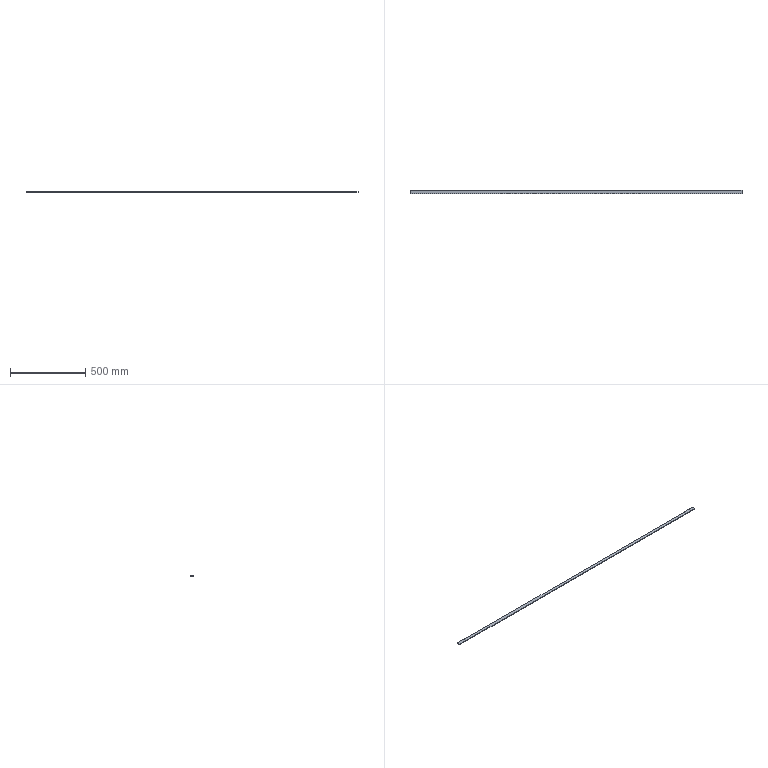Part | SolidWorks | features Chamfer 1, Extrusion 1, Fillet 1, ICE 1 | 1 solid | 12 faces | box 2200 x 24 x 4 mm | volume 178062 mm3 | plane 8 | cylinder 4 | commonest cylinder face diameters 4 x4
STEP:
#1=CARTESIAN_POINT('',(1030.,24.,0.));
#2=VERTEX_POINT('',#1);
#3=CARTESIAN_POINT('',(1100.,24.,0.));
#4=VERTEX_POINT('',#3);
#5=CARTESIAN_POINT('',(1100.,24.,0.));
#6=DIRECTION('',(1.,0.,0.));
#7=VECTOR('',#6,1000.);
#8=LINE('',#5,#7);
#9=EDGE_CURVE('',#2,#4,#8,.T.);
#10=ORIENTED_EDGE('',*,*,#9,.F.);
#11=CARTESIAN_POINT('',(1028.,22.,2.));
#12=VERTEX_POINT('',#11);
#13=CARTESIAN_POINT('',(1030.,24.,0.));
#14=CARTESIAN_POINT('',(1030.,24.,1.172));
#15=CARTESIAN_POINT('',(1029.172,23.172,2.));
#16=CARTESIAN_POINT('',(1028.,22.,2.));
#17=(BOUNDED_CURVE()B_SPLINE_CURVE(3,(#13,#14,#15,#16),.UNSPECIFIED.,.F.,.F.)B_SPLINE_CURVE_WITH_KNOTS((4,4),(3.142,4.712),.UNSPECIFIED.)CURVE()GEOMETRIC_REPRESENTATION_ITEM()RATIONAL_B_SPLINE_CURVE((1.,0.8047,0.8047,1.))REPRESENTATION_ITEM(''));
#18=EDGE_CURVE('',#2,#12,#17,.T.);
#19=ORIENTED_EDGE('',*,*,#18,.T.);
#20=CARTESIAN_POINT('',(1100.,22.,2.));
#21=VERTEX_POINT('',#20);
#22=CARTESIAN_POINT('',(-1100.,22.,2.));
#23=DIRECTION('',(-1.,0.,0.));
#24=VECTOR('',#23,1000.);
#25=LINE('',#22,#24);
#26=EDGE_CURVE('',#21,#12,#25,.T.);
#27=ORIENTED_EDGE('',*,*,#26,.F.);
#28=CARTESIAN_POINT('',(1100.,22.,0.));
#29=DIRECTION('',(1.,0.,0.));
#30=DIRECTION('',(0.,0.,1.));
#31=AXIS2_PLACEMENT_3D('',#28,#29,#30);
#32=CIRCLE('',#31,2.);
#33=EDGE_CURVE('',#4,#21,#32,.T.);
#34=ORIENTED_EDGE('',*,*,#33,.F.);
#35=EDGE_LOOP('',(#10,#19,#27,#34));
#36=FACE_OUTER_BOUND('',#35,.T.);
#37=CARTESIAN_POINT('',(0.,22.,0.));
#38=DIRECTION('',(-1.,0.,0.));
#39=DIRECTION('',(0.,0.,1.));
#40=AXIS2_PLACEMENT_3D('',#37,#38,#39);
#41=CYLINDRICAL_SURFACE('',#40,2.);
#42=ADVANCED_FACE('',(#36),#41,.T.);
#43=CARTESIAN_POINT('',(1028.,22.,-2.));
#44=VERTEX_POINT('',#43);
#45=CARTESIAN_POINT('',(1100.,22.,-2.));
#46=VERTEX_POINT('',#45);
#47=CARTESIAN_POINT('',(1100.,22.,-2.));
#48=DIRECTION('',(1.,0.,0.));
#49=VECTOR('',#48,1000.);
#50=LINE('',#47,#49);
#51=EDGE_CURVE('',#44,#46,#50,.T.);
#52=ORIENTED_EDGE('',*,*,#51,.F.);
#53=CARTESIAN_POINT('',(1028.,22.,-2.));
#54=CARTESIAN_POINT('',(1029.172,23.172,-2.));
#55=CARTESIAN_POINT('',(1030.,24.,-1.172));
#56=CARTESIAN_POINT('',(1030.,24.,0.));
#57=(BOUNDED_CURVE()B_SPLINE_CURVE(3,(#53,#54,#55,#56),.UNSPECIFIED.,.F.,.T.)B_SPLINE_CURVE_WITH_KNOTS((4,4),(4.712,6.283),.UNSPECIFIED.)CURVE()GEOMETRIC_REPRESENTATION_ITEM()RATIONAL_B_SPLINE_CURVE((1.,0.8047,0.8047,1.))REPRESENTATION_ITEM(''));
#58=EDGE_CURVE('',#44,#2,#57,.T.);
#59=ORIENTED_EDGE('',*,*,#58,.T.);
#60=ORIENTED_EDGE('',*,*,#9,.T.);
#61=CARTESIAN_POINT('',(1100.,22.,0.));
#62=DIRECTION('',(1.,0.,0.));
#63=DIRECTION('',(0.,0.,1.));
#64=AXIS2_PLACEMENT_3D('',#61,#62,#63);
#65=CIRCLE('',#64,2.);
#66=EDGE_CURVE('',#46,#4,#65,.T.);
#67=ORIENTED_EDGE('',*,*,#66,.F.);
#68=EDGE_LOOP('',(#52,#59,#60,#67));
#69=FACE_OUTER_BOUND('',#68,.T.);
#70=CARTESIAN_POINT('',(0.,22.,0.));
#71=DIRECTION('',(1.,0.,0.));
#72=DIRECTION('',(0.,0.,-1.));
#73=AXIS2_PLACEMENT_3D('',#70,#71,#72);
#74=CYLINDRICAL_SURFACE('',#73,2.);
#75=ADVANCED_FACE('',(#69),#74,.T.);
#76=CARTESIAN_POINT('',(-1100.,22.,2.));
#77=VERTEX_POINT('',#76);
#78=CARTESIAN_POINT('',(-1100.,24.,0.));
#79=VERTEX_POINT('',#78);
#80=CARTESIAN_POINT('',(-1100.,22.,0.));
#81=DIRECTION('',(-1.,0.,0.));
#82=DIRECTION('',(0.,0.,-1.));
#83=AXIS2_PLACEMENT_3D('',#80,#81,#82);
#84=CIRCLE('',#83,2.);
#85=EDGE_CURVE('',#77,#79,#84,.T.);
#86=ORIENTED_EDGE('',*,*,#85,.T.);
#87=CARTESIAN_POINT('',(-1100.,22.,-2.));
#88=VERTEX_POINT('',#87);
#89=CARTESIAN_POINT('',(-1100.,22.,0.));
#90=DIRECTION('',(-1.,0.,0.));
#91=DIRECTION('',(0.,0.,-1.));
#92=AXIS2_PLACEMENT_3D('',#89,#90,#91);
#93=CIRCLE('',#92,2.);
#94=EDGE_CURVE('',#79,#88,#93,.T.);
#95=ORIENTED_EDGE('',*,*,#94,.T.);
#96=CARTESIAN_POINT('',(-1100.,0.,-2.));
#97=VERTEX_POINT('',#96);
#98=CARTESIAN_POINT('',(-1100.,24.,-2.));
#99=DIRECTION('',(0.,-1.,0.));
#100=VECTOR('',#99,1000.);
#101=LINE('',#98,#100);
#102=EDGE_CURVE('',#88,#97,#101,.T.);
#103=ORIENTED_EDGE('',*,*,#102,.T.);
#104=CARTESIAN_POINT('',(-1100.,0.,2.));
#105=VERTEX_POINT('',#104);
#106=CARTESIAN_POINT('',(-1100.,0.,2.));
#107=DIRECTION('',(0.,0.,1.));
#108=VECTOR('',#107,1000.);
#109=LINE('',#106,#108);
#110=EDGE_CURVE('',#97,#105,#109,.T.);
#111=ORIENTED_EDGE('',*,*,#110,.T.);
#112=CARTESIAN_POINT('',(-1100.,24.,2.));
#113=DIRECTION('',(0.,-1.,0.));
#114=VECTOR('',#113,1000.);
#115=LINE('',#112,#114);
#116=EDGE_CURVE('',#77,#105,#115,.T.);
#117=ORIENTED_EDGE('',*,*,#116,.F.);
#118=EDGE_LOOP('',(#86,#95,#103,#111,#117));
#119=FACE_OUTER_BOUND('',#118,.T.);
#120=CARTESIAN_POINT('',(-1100.,24.,2.));
#121=DIRECTION('',(1.,0.,0.));
#122=DIRECTION('',(0.,0.,-1.));
#123=AXIS2_PLACEMENT_3D('',#120,#121,#122);
#124=PLANE('',#123);
#125=ADVANCED_FACE('',(#119),#124,.F.);
#126=ORIENTED_EDGE('',*,*,#26,.T.);
#127=CARTESIAN_POINT('',(1026.,20.,2.));
#128=VERTEX_POINT('',#127);
#129=CARTESIAN_POINT('',(1065.,59.,2.));
#130=DIRECTION('',(-0.7071,-0.7071,0.));
#131=VECTOR('',#130,1000.);
#132=LINE('',#129,#131);
#133=EDGE_CURVE('',#12,#128,#132,.T.);
#134=ORIENTED_EDGE('',*,*,#133,.T.);
#135=CARTESIAN_POINT('',(-1026.,20.,2.));
#136=VERTEX_POINT('',#135);
#137=CARTESIAN_POINT('',(-1030.,20.,2.));
#138=DIRECTION('',(1.,0.,0.));
#139=VECTOR('',#138,1000.);
#140=LINE('',#137,#139);
#141=EDGE_CURVE('',#136,#128,#140,.T.);
#142=ORIENTED_EDGE('',*,*,#141,.F.);
#143=CARTESIAN_POINT('',(-1028.,22.,2.));
#144=VERTEX_POINT('',#143);
#145=CARTESIAN_POINT('',(35.,-1041.,2.));
#146=DIRECTION('',(-0.7071,0.7071,0.));
#147=VECTOR('',#146,1000.);
#148=LINE('',#145,#147);
#149=EDGE_CURVE('',#136,#144,#148,.T.);
#150=ORIENTED_EDGE('',*,*,#149,.T.);
#151=CARTESIAN_POINT('',(-1100.,22.,2.));
#152=DIRECTION('',(-1.,0.,0.));
#153=VECTOR('',#152,1000.);
#154=LINE('',#151,#153);
#155=EDGE_CURVE('',#144,#77,#154,.T.);
#156=ORIENTED_EDGE('',*,*,#155,.T.);
#157=ORIENTED_EDGE('',*,*,#116,.T.);
#158=CARTESIAN_POINT('',(1100.,0.,2.));
#159=VERTEX_POINT('',#158);
#160=CARTESIAN_POINT('',(1100.,0.,2.));
#161=DIRECTION('',(1.,0.,0.));
#162=VECTOR('',#161,1000.);
#163=LINE('',#160,#162);
#164=EDGE_CURVE('',#105,#159,#163,.T.);
#165=ORIENTED_EDGE('',*,*,#164,.T.);
#166=CARTESIAN_POINT('',(1100.,24.,2.));
#167=DIRECTION('',(0.,-1.,0.));
#168=VECTOR('',#167,1000.);
#169=LINE('',#166,#168);
#170=EDGE_CURVE('',#21,#159,#169,.T.);
#171=ORIENTED_EDGE('',*,*,#170,.F.);
#172=EDGE_LOOP('',(#126,#134,#142,#150,#156,#157,#165,#171));
#173=FACE_OUTER_BOUND('',#172,.T.);
#174=CARTESIAN_POINT('',(1100.,24.,2.));
#175=DIRECTION('',(0.,0.,-1.));
#176=DIRECTION('',(-1.,0.,0.));
#177=AXIS2_PLACEMENT_3D('',#174,#175,#176);
#178=PLANE('',#177);
#179=ADVANCED_FACE('',(#173),#178,.F.);
#180=CARTESIAN_POINT('',(1100.,0.,-2.));
#181=VERTEX_POINT('',#180);
#182=CARTESIAN_POINT('',(1100.,24.,-2.));
#183=DIRECTION('',(0.,-1.,0.));
#184=VECTOR('',#183,1000.);
#185=LINE('',#182,#184);
#186=EDGE_CURVE('',#46,#181,#185,.T.);
#187=ORIENTED_EDGE('',*,*,#186,.F.);
#188=ORIENTED_EDGE('',*,*,#66,.T.);
#189=ORIENTED_EDGE('',*,*,#33,.T.);
#190=ORIENTED_EDGE('',*,*,#170,.T.);
#191=CARTESIAN_POINT('',(1100.,0.,2.));
#192=DIRECTION('',(0.,0.,-1.));
#193=VECTOR('',#192,1000.);
#194=LINE('',#191,#193);
#195=EDGE_CURVE('',#159,#181,#194,.T.);
#196=ORIENTED_EDGE('',*,*,#195,.T.);
#197=EDGE_LOOP('',(#187,#188,#189,#190,#196));
#198=FACE_OUTER_BOUND('',#197,.T.);
#199=CARTESIAN_POINT('',(1100.,24.,2.));
#200=DIRECTION('',(-1.,0.,0.));
#201=DIRECTION('',(0.,0.,1.));
#202=AXIS2_PLACEMENT_3D('',#199,#200,#201);
#203=PLANE('',#202);
#204=ADVANCED_FACE('',(#198),#203,.F.);
#205=CARTESIAN_POINT('',(-1028.,22.,-2.));
#206=VERTEX_POINT('',#205);
#207=CARTESIAN_POINT('',(1100.,22.,-2.));
#208=DIRECTION('',(1.,0.,0.));
#209=VECTOR('',#208,1000.);
#210=LINE('',#207,#209);
#211=EDGE_CURVE('',#88,#206,#210,.T.);
#212=ORIENTED_EDGE('',*,*,#211,.T.);
#213=CARTESIAN_POINT('',(-1026.,20.,-2.));
#214=VERTEX_POINT('',#213);
#215=CARTESIAN_POINT('',(35.,-1041.,-2.));
#216=DIRECTION('',(0.7071,-0.7071,0.));
#217=VECTOR('',#216,1000.);
#218=LINE('',#215,#217);
#219=EDGE_CURVE('',#206,#214,#218,.T.);
#220=ORIENTED_EDGE('',*,*,#219,.T.);
#221=CARTESIAN_POINT('',(1026.,20.,-2.));
#222=VERTEX_POINT('',#221);
#223=CARTESIAN_POINT('',(-1030.,20.,-2.));
#224=DIRECTION('',(1.,0.,0.));
#225=VECTOR('',#224,1000.);
#226=LINE('',#223,#225);
#227=EDGE_CURVE('',#214,#222,#226,.T.);
#228=ORIENTED_EDGE('',*,*,#227,.T.);
#229=CARTESIAN_POINT('',(1065.,59.,-2.));
#230=DIRECTION('',(0.7071,0.7071,0.));
#231=VECTOR('',#230,1000.);
#232=LINE('',#229,#231);
#233=EDGE_CURVE('',#222,#44,#232,.T.);
#234=ORIENTED_EDGE('',*,*,#233,.T.);
#235=ORIENTED_EDGE('',*,*,#51,.T.);
#236=ORIENTED_EDGE('',*,*,#186,.T.);
#237=CARTESIAN_POINT('',(1100.,0.,-2.));
#238=DIRECTION('',(-1.,0.,0.));
#239=VECTOR('',#238,1000.);
#240=LINE('',#237,#239);
#241=EDGE_CURVE('',#181,#97,#240,.T.);
#242=ORIENTED_EDGE('',*,*,#241,.T.);
#243=ORIENTED_EDGE('',*,*,#102,.F.);
#244=EDGE_LOOP('',(#212,#220,#228,#234,#235,#236,#242,#243));
#245=FACE_OUTER_BOUND('',#244,.T.);
#246=CARTESIAN_POINT('',(1100.,24.,-2.));
#247=DIRECTION('',(0.,0.,1.));
#248=DIRECTION('',(1.,0.,0.));
#249=AXIS2_PLACEMENT_3D('',#246,#247,#248);
#250=PLANE('',#249);
#251=ADVANCED_FACE('',(#245),#250,.F.);
#252=ORIENTED_EDGE('',*,*,#110,.F.);
#253=ORIENTED_EDGE('',*,*,#241,.F.);
#254=ORIENTED_EDGE('',*,*,#195,.F.);
#255=ORIENTED_EDGE('',*,*,#164,.F.);
#256=EDGE_LOOP('',(#252,#253,#254,#255));
#257=FACE_OUTER_BOUND('',#256,.T.);
#258=CARTESIAN_POINT('',(0.,0.,0.));
#259=DIRECTION('',(0.,1.,0.));
#260=DIRECTION('',(0.,0.,1.));
#261=AXIS2_PLACEMENT_3D('',#258,#259,#260);
#262=PLANE('',#261);
#263=ADVANCED_FACE('',(#257),#262,.F.);
#264=ORIENTED_EDGE('',*,*,#155,.F.);
#265=CARTESIAN_POINT('',(-1030.,24.,0.));
#266=VERTEX_POINT('',#265);
#267=CARTESIAN_POINT('',(-1028.,22.,2.));
#268=CARTESIAN_POINT('',(-1029.172,23.172,2.));
#269=CARTESIAN_POINT('',(-1030.,24.,1.172));
#270=CARTESIAN_POINT('',(-1030.,24.,0.));
#271=(BOUNDED_CURVE()B_SPLINE_CURVE(3,(#267,#268,#269,#270),.UNSPECIFIED.,.F.,.F.)B_SPLINE_CURVE_WITH_KNOTS((4,4),(4.712,6.283),.UNSPECIFIED.)CURVE()GEOMETRIC_REPRESENTATION_ITEM()RATIONAL_B_SPLINE_CURVE((1.,0.8047,0.8047,1.))REPRESENTATION_ITEM(''));
#272=EDGE_CURVE('',#144,#266,#271,.T.);
#273=ORIENTED_EDGE('',*,*,#272,.T.);
#274=CARTESIAN_POINT('',(1100.,24.,0.));
#275=DIRECTION('',(1.,0.,0.));
#276=VECTOR('',#275,1000.);
#277=LINE('',#274,#276);
#278=EDGE_CURVE('',#79,#266,#277,.T.);
#279=ORIENTED_EDGE('',*,*,#278,.F.);
#280=ORIENTED_EDGE('',*,*,#85,.F.);
#281=EDGE_LOOP('',(#264,#273,#279,#280));
#282=FACE_OUTER_BOUND('',#281,.T.);
#283=CARTESIAN_POINT('',(0.,22.,0.));
#284=DIRECTION('',(-1.,0.,0.));
#285=DIRECTION('',(0.,0.,1.));
#286=AXIS2_PLACEMENT_3D('',#283,#284,#285);
#287=CYLINDRICAL_SURFACE('',#286,2.);
#288=ADVANCED_FACE('',(#282),#287,.T.);
#289=ORIENTED_EDGE('',*,*,#278,.T.);
#290=CARTESIAN_POINT('',(-1030.,24.,0.));
#291=CARTESIAN_POINT('',(-1030.,24.,-1.172));
#292=CARTESIAN_POINT('',(-1029.172,23.172,-2.));
#293=CARTESIAN_POINT('',(-1028.,22.,-2.));
#294=(BOUNDED_CURVE()B_SPLINE_CURVE(3,(#290,#291,#292,#293),.UNSPECIFIED.,.F.,.F.)B_SPLINE_CURVE_WITH_KNOTS((4,4),(3.142,4.712),.UNSPECIFIED.)CURVE()GEOMETRIC_REPRESENTATION_ITEM()RATIONAL_B_SPLINE_CURVE((1.,0.8047,0.8047,1.))REPRESENTATION_ITEM(''));
#295=EDGE_CURVE('',#266,#206,#294,.T.);
#296=ORIENTED_EDGE('',*,*,#295,.T.);
#297=ORIENTED_EDGE('',*,*,#211,.F.);
#298=ORIENTED_EDGE('',*,*,#94,.F.);
#299=EDGE_LOOP('',(#289,#296,#297,#298));
#300=FACE_OUTER_BOUND('',#299,.T.);
#301=CARTESIAN_POINT('',(0.,22.,0.));
#302=DIRECTION('',(1.,0.,0.));
#303=DIRECTION('',(0.,0.,-1.));
#304=AXIS2_PLACEMENT_3D('',#301,#302,#303);
#305=CYLINDRICAL_SURFACE('',#304,2.);
#306=ADVANCED_FACE('',(#300),#305,.T.);
#307=ORIENTED_EDGE('',*,*,#141,.T.);
#308=CARTESIAN_POINT('',(1026.,20.,-2.));
#309=DIRECTION('',(0.,0.,-1.));
#310=VECTOR('',#309,1000.);
#311=LINE('',#308,#310);
#312=EDGE_CURVE('',#128,#222,#311,.T.);
#313=ORIENTED_EDGE('',*,*,#312,.T.);
#314=ORIENTED_EDGE('',*,*,#227,.F.);
#315=CARTESIAN_POINT('',(-1026.,20.,2.));
#316=DIRECTION('',(0.,0.,1.));
#317=VECTOR('',#316,1000.);
#318=LINE('',#315,#317);
#319=EDGE_CURVE('',#214,#136,#318,.T.);
#320=ORIENTED_EDGE('',*,*,#319,.T.);
#321=EDGE_LOOP('',(#307,#313,#314,#320));
#322=FACE_OUTER_BOUND('',#321,.T.);
#323=CARTESIAN_POINT('',(-1030.,20.,-2.));
#324=DIRECTION('',(0.,-1.,0.));
#325=DIRECTION('',(0.,0.,-1.));
#326=AXIS2_PLACEMENT_3D('',#323,#324,#325);
#327=PLANE('',#326);
#328=ADVANCED_FACE('',(#322),#327,.F.);
#329=ORIENTED_EDGE('',*,*,#233,.F.);
#330=ORIENTED_EDGE('',*,*,#312,.F.);
#331=ORIENTED_EDGE('',*,*,#133,.F.);
#332=ORIENTED_EDGE('',*,*,#18,.F.);
#333=ORIENTED_EDGE('',*,*,#58,.F.);
#334=EDGE_LOOP('',(#329,#330,#331,#332,#333));
#335=FACE_OUTER_BOUND('',#334,.T.);
#336=CARTESIAN_POINT('',(1030.,24.,-2.));
#337=DIRECTION('',(-0.7071,0.7071,0.));
#338=DIRECTION('',(0.,0.,-1.));
#339=AXIS2_PLACEMENT_3D('',#336,#337,#338);
#340=PLANE('',#339);
#341=ADVANCED_FACE('',(#335),#340,.T.);
#342=ORIENTED_EDGE('',*,*,#219,.F.);
#343=ORIENTED_EDGE('',*,*,#295,.F.);
#344=ORIENTED_EDGE('',*,*,#272,.F.);
#345=ORIENTED_EDGE('',*,*,#149,.F.);
#346=ORIENTED_EDGE('',*,*,#319,.F.);
#347=EDGE_LOOP('',(#342,#343,#344,#345,#346));
#348=FACE_OUTER_BOUND('',#347,.T.);
#349=CARTESIAN_POINT('',(-1026.,20.,-2.));
#350=DIRECTION('',(0.7071,0.7071,0.));
#351=DIRECTION('',(0.,0.,-1.));
#352=AXIS2_PLACEMENT_3D('',#349,#350,#351);
#353=PLANE('',#352);
#354=ADVANCED_FACE('',(#348),#353,.T.);
#355=CLOSED_SHELL('',(#42,#75,#125,#179,#204,#251,#263,#288,#306,#328,#341,#354));
#356=MANIFOLD_SOLID_BREP('',#355);
#357=CARTESIAN_POINT('',(0.,0.,0.));
#358=DIRECTION('',(0.,0.,1.));
#359=DIRECTION('',(1.,0.,0.));
#360=AXIS2_PLACEMENT_3D('',#357,#358,#359);
#361=(LENGTH_UNIT()NAMED_UNIT(*)SI_UNIT(.MILLI.,.METRE.));
#362=UNCERTAINTY_MEASURE_WITH_UNIT(LENGTH_MEASURE(0.00001),#361,'','');
#363=(NAMED_UNIT(*)PLANE_ANGLE_UNIT()SI_UNIT($,.RADIAN.));
#364=(NAMED_UNIT(*)SI_UNIT($,.STERADIAN.)SOLID_ANGLE_UNIT());
#365=(GEOMETRIC_REPRESENTATION_CONTEXT(3)GLOBAL_UNCERTAINTY_ASSIGNED_CONTEXT((#362))GLOBAL_UNIT_ASSIGNED_CONTEXT((#361,#363,#364))REPRESENTATION_CONTEXT('',''));
#366=ADVANCED_BREP_SHAPE_REPRESENTATION('',(#356,#360),#365);